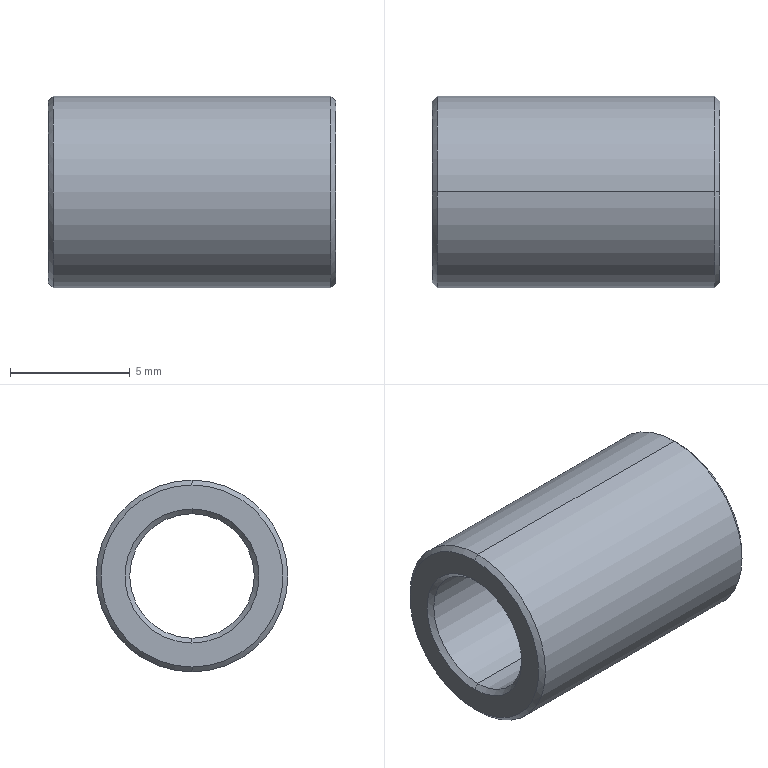Part | NX | features BREP 1 | 1 solid | 14 faces | box 12 x 8 x 8 mm | volume 346.681 mm3 | cone 8 | cylinder 4 | plane 2 | commonest cylinder face diameters 5.2 x2 8 x2
STEP:
#1=CARTESIAN_POINT('',(11.8,0.,-4.));
#2=VERTEX_POINT('',#1);
#3=CARTESIAN_POINT('',(12.,0.,-3.8));
#4=VERTEX_POINT('',#3);
#5=CARTESIAN_POINT('',(12.,0.,-3.8));
#6=DIRECTION('',(-0.7071,0.,-0.7071));
#7=VECTOR('',#6,1000.);
#8=LINE('',#5,#7);
#9=EDGE_CURVE('',#2,#4,#8,.F.);
#10=ORIENTED_EDGE('',*,*,#9,.T.);
#11=CARTESIAN_POINT('',(12.,0.,3.8));
#12=VERTEX_POINT('',#11);
#13=CARTESIAN_POINT('',(12.,0.,0.));
#14=DIRECTION('',(1.,0.,0.));
#15=DIRECTION('',(0.,0.,-1.));
#16=AXIS2_PLACEMENT_3D('',#13,#14,#15);
#17=CIRCLE('',#16,3.8);
#18=EDGE_CURVE('',#12,#4,#17,.T.);
#19=ORIENTED_EDGE('',*,*,#18,.F.);
#20=CARTESIAN_POINT('',(11.8,0.,4.));
#21=VERTEX_POINT('',#20);
#22=CARTESIAN_POINT('',(12.,0.,3.8));
#23=DIRECTION('',(-0.7071,0.,0.7071));
#24=VECTOR('',#23,1000.);
#25=LINE('',#22,#24);
#26=EDGE_CURVE('',#21,#12,#25,.F.);
#27=ORIENTED_EDGE('',*,*,#26,.F.);
#28=CARTESIAN_POINT('',(11.8,0.,0.));
#29=DIRECTION('',(-1.,0.,0.));
#30=DIRECTION('',(0.,0.,-1.));
#31=AXIS2_PLACEMENT_3D('',#28,#29,#30);
#32=CIRCLE('',#31,4.);
#33=EDGE_CURVE('',#2,#21,#32,.T.);
#34=ORIENTED_EDGE('',*,*,#33,.F.);
#35=EDGE_LOOP('',(#10,#19,#27,#34));
#36=FACE_BOUND('',#35,.T.);
#37=CARTESIAN_POINT('',(12.,0.,0.));
#38=DIRECTION('',(-1.,0.,0.));
#39=DIRECTION('',(0.,0.,1.));
#40=AXIS2_PLACEMENT_3D('',#37,#38,#39);
#41=CONICAL_SURFACE('',#40,3.8,0.7854);
#42=ADVANCED_FACE('',(#36),#41,.T.);
#43=CARTESIAN_POINT('',(11.8,0.,2.6));
#44=VERTEX_POINT('',#43);
#45=CARTESIAN_POINT('',(12.,0.,2.8));
#46=VERTEX_POINT('',#45);
#47=CARTESIAN_POINT('',(11.8,0.,2.6));
#48=DIRECTION('',(0.7071,0.,0.7071));
#49=VECTOR('',#48,1000.);
#50=LINE('',#47,#49);
#51=EDGE_CURVE('',#44,#46,#50,.T.);
#52=ORIENTED_EDGE('',*,*,#51,.F.);
#53=CARTESIAN_POINT('',(11.8,0.,-2.6));
#54=VERTEX_POINT('',#53);
#55=CARTESIAN_POINT('',(11.8,0.,0.));
#56=DIRECTION('',(1.,0.,0.));
#57=DIRECTION('',(0.,0.,-1.));
#58=AXIS2_PLACEMENT_3D('',#55,#56,#57);
#59=CIRCLE('',#58,2.6);
#60=EDGE_CURVE('',#54,#44,#59,.T.);
#61=ORIENTED_EDGE('',*,*,#60,.F.);
#62=CARTESIAN_POINT('',(12.,0.,-2.8));
#63=VERTEX_POINT('',#62);
#64=CARTESIAN_POINT('',(11.8,0.,-2.6));
#65=DIRECTION('',(0.7071,0.,-0.7071));
#66=VECTOR('',#65,1000.);
#67=LINE('',#64,#66);
#68=EDGE_CURVE('',#54,#63,#67,.T.);
#69=ORIENTED_EDGE('',*,*,#68,.T.);
#70=CARTESIAN_POINT('',(12.,0.,0.));
#71=DIRECTION('',(-1.,0.,0.));
#72=DIRECTION('',(0.,0.,-1.));
#73=AXIS2_PLACEMENT_3D('',#70,#71,#72);
#74=CIRCLE('',#73,2.8);
#75=EDGE_CURVE('',#46,#63,#74,.T.);
#76=ORIENTED_EDGE('',*,*,#75,.F.);
#77=EDGE_LOOP('',(#52,#61,#69,#76));
#78=FACE_BOUND('',#77,.T.);
#79=CARTESIAN_POINT('',(11.8,0.,0.));
#80=DIRECTION('',(1.,0.,0.));
#81=DIRECTION('',(0.,0.,-1.));
#82=AXIS2_PLACEMENT_3D('',#79,#80,#81);
#83=CONICAL_SURFACE('',#82,2.6,0.7854);
#84=ADVANCED_FACE('',(#78),#83,.F.);
#85=CARTESIAN_POINT('',(0.,0.,3.8));
#86=VERTEX_POINT('',#85);
#87=CARTESIAN_POINT('',(0.2,0.,4.));
#88=VERTEX_POINT('',#87);
#89=CARTESIAN_POINT('',(0.2,0.,4.));
#90=DIRECTION('',(0.7071,0.,0.7071));
#91=VECTOR('',#90,1000.);
#92=LINE('',#89,#91);
#93=EDGE_CURVE('',#86,#88,#92,.T.);
#94=ORIENTED_EDGE('',*,*,#93,.F.);
#95=CARTESIAN_POINT('',(0.,0.,-3.8));
#96=VERTEX_POINT('',#95);
#97=CARTESIAN_POINT('',(0.,0.,0.));
#98=DIRECTION('',(-1.,0.,0.));
#99=DIRECTION('',(0.,0.,-1.));
#100=AXIS2_PLACEMENT_3D('',#97,#98,#99);
#101=CIRCLE('',#100,3.8);
#102=EDGE_CURVE('',#96,#86,#101,.T.);
#103=ORIENTED_EDGE('',*,*,#102,.F.);
#104=CARTESIAN_POINT('',(0.2,0.,-4.));
#105=VERTEX_POINT('',#104);
#106=CARTESIAN_POINT('',(0.2,0.,-4.));
#107=DIRECTION('',(0.7071,0.,-0.7071));
#108=VECTOR('',#107,1000.);
#109=LINE('',#106,#108);
#110=EDGE_CURVE('',#96,#105,#109,.T.);
#111=ORIENTED_EDGE('',*,*,#110,.T.);
#112=CARTESIAN_POINT('',(0.2,0.,0.));
#113=DIRECTION('',(1.,0.,0.));
#114=DIRECTION('',(0.,0.,-1.));
#115=AXIS2_PLACEMENT_3D('',#112,#113,#114);
#116=CIRCLE('',#115,4.);
#117=EDGE_CURVE('',#88,#105,#116,.T.);
#118=ORIENTED_EDGE('',*,*,#117,.F.);
#119=EDGE_LOOP('',(#94,#103,#111,#118));
#120=FACE_BOUND('',#119,.T.);
#121=CARTESIAN_POINT('',(0.2,0.,0.));
#122=DIRECTION('',(1.,0.,0.));
#123=DIRECTION('',(0.,0.,-1.));
#124=AXIS2_PLACEMENT_3D('',#121,#122,#123);
#125=CONICAL_SURFACE('',#124,4.,0.7854);
#126=ADVANCED_FACE('',(#120),#125,.T.);
#127=CARTESIAN_POINT('',(0.,0.,-2.8));
#128=VERTEX_POINT('',#127);
#129=CARTESIAN_POINT('',(0.2,0.,-2.6));
#130=VERTEX_POINT('',#129);
#131=CARTESIAN_POINT('',(0.,0.,-2.8));
#132=DIRECTION('',(-0.7071,0.,-0.7071));
#133=VECTOR('',#132,1000.);
#134=LINE('',#131,#133);
#135=EDGE_CURVE('',#128,#130,#134,.F.);
#136=ORIENTED_EDGE('',*,*,#135,.T.);
#137=CARTESIAN_POINT('',(0.2,0.,2.6));
#138=VERTEX_POINT('',#137);
#139=CARTESIAN_POINT('',(0.2,0.,0.));
#140=DIRECTION('',(-1.,0.,0.));
#141=DIRECTION('',(0.,0.,-1.));
#142=AXIS2_PLACEMENT_3D('',#139,#140,#141);
#143=CIRCLE('',#142,2.6);
#144=EDGE_CURVE('',#138,#130,#143,.T.);
#145=ORIENTED_EDGE('',*,*,#144,.F.);
#146=CARTESIAN_POINT('',(0.,0.,2.8));
#147=VERTEX_POINT('',#146);
#148=CARTESIAN_POINT('',(0.,0.,2.8));
#149=DIRECTION('',(-0.7071,0.,0.7071));
#150=VECTOR('',#149,1000.);
#151=LINE('',#148,#150);
#152=EDGE_CURVE('',#147,#138,#151,.F.);
#153=ORIENTED_EDGE('',*,*,#152,.F.);
#154=CARTESIAN_POINT('',(0.,0.,0.));
#155=DIRECTION('',(1.,0.,0.));
#156=DIRECTION('',(0.,0.,-1.));
#157=AXIS2_PLACEMENT_3D('',#154,#155,#156);
#158=CIRCLE('',#157,2.8);
#159=EDGE_CURVE('',#128,#147,#158,.T.);
#160=ORIENTED_EDGE('',*,*,#159,.F.);
#161=EDGE_LOOP('',(#136,#145,#153,#160));
#162=FACE_BOUND('',#161,.T.);
#163=CARTESIAN_POINT('',(0.,0.,0.));
#164=DIRECTION('',(-1.,0.,0.));
#165=DIRECTION('',(0.,0.,1.));
#166=AXIS2_PLACEMENT_3D('',#163,#164,#165);
#167=CONICAL_SURFACE('',#166,2.8,0.7854);
#168=ADVANCED_FACE('',(#162),#167,.F.);
#169=CARTESIAN_POINT('',(12.,0.,-2.6));
#170=DIRECTION('',(-1.,0.,0.));
#171=VECTOR('',#170,1000.);
#172=LINE('',#169,#171);
#173=EDGE_CURVE('',#130,#54,#172,.F.);
#174=ORIENTED_EDGE('',*,*,#173,.T.);
#175=ORIENTED_EDGE('',*,*,#60,.T.);
#176=CARTESIAN_POINT('',(12.,0.,2.6));
#177=DIRECTION('',(-1.,0.,0.));
#178=VECTOR('',#177,1000.);
#179=LINE('',#176,#178);
#180=EDGE_CURVE('',#138,#44,#179,.F.);
#181=ORIENTED_EDGE('',*,*,#180,.F.);
#182=ORIENTED_EDGE('',*,*,#144,.T.);
#183=EDGE_LOOP('',(#174,#175,#181,#182));
#184=FACE_BOUND('',#183,.T.);
#185=CARTESIAN_POINT('',(12.,0.,0.));
#186=DIRECTION('',(-1.,0.,0.));
#187=DIRECTION('',(0.,0.,1.));
#188=AXIS2_PLACEMENT_3D('',#185,#186,#187);
#189=CYLINDRICAL_SURFACE('',#188,2.6);
#190=ADVANCED_FACE('',(#184),#189,.F.);
#191=CARTESIAN_POINT('',(12.,0.,-4.));
#192=DIRECTION('',(-1.,0.,0.));
#193=VECTOR('',#192,1000.);
#194=LINE('',#191,#193);
#195=EDGE_CURVE('',#105,#2,#194,.F.);
#196=ORIENTED_EDGE('',*,*,#195,.T.);
#197=ORIENTED_EDGE('',*,*,#33,.T.);
#198=CARTESIAN_POINT('',(12.,0.,4.));
#199=DIRECTION('',(-1.,0.,0.));
#200=VECTOR('',#199,1000.);
#201=LINE('',#198,#200);
#202=EDGE_CURVE('',#88,#21,#201,.F.);
#203=ORIENTED_EDGE('',*,*,#202,.F.);
#204=ORIENTED_EDGE('',*,*,#117,.T.);
#205=EDGE_LOOP('',(#196,#197,#203,#204));
#206=FACE_BOUND('',#205,.T.);
#207=CARTESIAN_POINT('',(12.,0.,0.));
#208=DIRECTION('',(-1.,0.,0.));
#209=DIRECTION('',(0.,0.,1.));
#210=AXIS2_PLACEMENT_3D('',#207,#208,#209);
#211=CYLINDRICAL_SURFACE('',#210,4.);
#212=ADVANCED_FACE('',(#206),#211,.T.);
#213=ORIENTED_EDGE('',*,*,#102,.T.);
#214=CARTESIAN_POINT('',(0.,0.,0.));
#215=DIRECTION('',(-1.,0.,0.));
#216=DIRECTION('',(0.,0.,-1.));
#217=AXIS2_PLACEMENT_3D('',#214,#215,#216);
#218=CIRCLE('',#217,3.8);
#219=EDGE_CURVE('',#86,#96,#218,.T.);
#220=ORIENTED_EDGE('',*,*,#219,.T.);
#221=EDGE_LOOP('',(#213,#220));
#222=FACE_BOUND('',#221,.T.);
#223=CARTESIAN_POINT('',(0.,0.,0.));
#224=DIRECTION('',(1.,0.,0.));
#225=DIRECTION('',(0.,0.,-1.));
#226=AXIS2_PLACEMENT_3D('',#223,#224,#225);
#227=CIRCLE('',#226,2.8);
#228=EDGE_CURVE('',#147,#128,#227,.T.);
#229=ORIENTED_EDGE('',*,*,#228,.T.);
#230=ORIENTED_EDGE('',*,*,#159,.T.);
#231=EDGE_LOOP('',(#229,#230));
#232=FACE_BOUND('',#231,.T.);
#233=CARTESIAN_POINT('',(0.,0.,0.));
#234=DIRECTION('',(1.,0.,0.));
#235=DIRECTION('',(0.,0.,-1.));
#236=AXIS2_PLACEMENT_3D('',#233,#234,#235);
#237=PLANE('',#236);
#238=ADVANCED_FACE('',(#222,#232),#237,.F.);
#239=ORIENTED_EDGE('',*,*,#18,.T.);
#240=CARTESIAN_POINT('',(12.,0.,0.));
#241=DIRECTION('',(1.,0.,0.));
#242=DIRECTION('',(0.,0.,-1.));
#243=AXIS2_PLACEMENT_3D('',#240,#241,#242);
#244=CIRCLE('',#243,3.8);
#245=EDGE_CURVE('',#4,#12,#244,.T.);
#246=ORIENTED_EDGE('',*,*,#245,.T.);
#247=EDGE_LOOP('',(#239,#246));
#248=FACE_BOUND('',#247,.T.);
#249=CARTESIAN_POINT('',(12.,0.,0.));
#250=DIRECTION('',(-1.,0.,0.));
#251=DIRECTION('',(0.,0.,-1.));
#252=AXIS2_PLACEMENT_3D('',#249,#250,#251);
#253=CIRCLE('',#252,2.8);
#254=EDGE_CURVE('',#63,#46,#253,.T.);
#255=ORIENTED_EDGE('',*,*,#254,.T.);
#256=ORIENTED_EDGE('',*,*,#75,.T.);
#257=EDGE_LOOP('',(#255,#256));
#258=FACE_BOUND('',#257,.T.);
#259=CARTESIAN_POINT('',(12.,0.,0.));
#260=DIRECTION('',(1.,0.,0.));
#261=DIRECTION('',(0.,0.,-1.));
#262=AXIS2_PLACEMENT_3D('',#259,#260,#261);
#263=PLANE('',#262);
#264=ADVANCED_FACE('',(#248,#258),#263,.T.);
#265=CARTESIAN_POINT('',(11.8,0.,0.));
#266=DIRECTION('',(-1.,0.,0.));
#267=DIRECTION('',(0.,0.,-1.));
#268=AXIS2_PLACEMENT_3D('',#265,#266,#267);
#269=CIRCLE('',#268,4.);
#270=EDGE_CURVE('',#21,#2,#269,.T.);
#271=ORIENTED_EDGE('',*,*,#270,.T.);
#272=ORIENTED_EDGE('',*,*,#195,.F.);
#273=CARTESIAN_POINT('',(0.2,0.,0.));
#274=DIRECTION('',(1.,0.,0.));
#275=DIRECTION('',(0.,0.,-1.));
#276=AXIS2_PLACEMENT_3D('',#273,#274,#275);
#277=CIRCLE('',#276,4.);
#278=EDGE_CURVE('',#105,#88,#277,.T.);
#279=ORIENTED_EDGE('',*,*,#278,.T.);
#280=ORIENTED_EDGE('',*,*,#202,.T.);
#281=EDGE_LOOP('',(#271,#272,#279,#280));
#282=FACE_BOUND('',#281,.T.);
#283=CARTESIAN_POINT('',(12.,0.,0.));
#284=DIRECTION('',(-1.,0.,0.));
#285=DIRECTION('',(0.,0.,1.));
#286=AXIS2_PLACEMENT_3D('',#283,#284,#285);
#287=CYLINDRICAL_SURFACE('',#286,4.);
#288=ADVANCED_FACE('',(#282),#287,.T.);
#289=CARTESIAN_POINT('',(11.8,0.,0.));
#290=DIRECTION('',(1.,0.,0.));
#291=DIRECTION('',(0.,0.,-1.));
#292=AXIS2_PLACEMENT_3D('',#289,#290,#291);
#293=CIRCLE('',#292,2.6);
#294=EDGE_CURVE('',#44,#54,#293,.T.);
#295=ORIENTED_EDGE('',*,*,#294,.T.);
#296=ORIENTED_EDGE('',*,*,#173,.F.);
#297=CARTESIAN_POINT('',(0.2,0.,0.));
#298=DIRECTION('',(-1.,0.,0.));
#299=DIRECTION('',(0.,0.,-1.));
#300=AXIS2_PLACEMENT_3D('',#297,#298,#299);
#301=CIRCLE('',#300,2.6);
#302=EDGE_CURVE('',#130,#138,#301,.T.);
#303=ORIENTED_EDGE('',*,*,#302,.T.);
#304=ORIENTED_EDGE('',*,*,#180,.T.);
#305=EDGE_LOOP('',(#295,#296,#303,#304));
#306=FACE_BOUND('',#305,.T.);
#307=CARTESIAN_POINT('',(12.,0.,0.));
#308=DIRECTION('',(-1.,0.,0.));
#309=DIRECTION('',(0.,0.,1.));
#310=AXIS2_PLACEMENT_3D('',#307,#308,#309);
#311=CYLINDRICAL_SURFACE('',#310,2.6);
#312=ADVANCED_FACE('',(#306),#311,.F.);
#313=ORIENTED_EDGE('',*,*,#302,.F.);
#314=ORIENTED_EDGE('',*,*,#135,.F.);
#315=ORIENTED_EDGE('',*,*,#228,.F.);
#316=ORIENTED_EDGE('',*,*,#152,.T.);
#317=EDGE_LOOP('',(#313,#314,#315,#316));
#318=FACE_BOUND('',#317,.T.);
#319=CARTESIAN_POINT('',(0.,0.,0.));
#320=DIRECTION('',(-1.,0.,0.));
#321=DIRECTION('',(0.,0.,1.));
#322=AXIS2_PLACEMENT_3D('',#319,#320,#321);
#323=CONICAL_SURFACE('',#322,2.8,0.7854);
#324=ADVANCED_FACE('',(#318),#323,.F.);
#325=ORIENTED_EDGE('',*,*,#219,.F.);
#326=ORIENTED_EDGE('',*,*,#93,.T.);
#327=ORIENTED_EDGE('',*,*,#278,.F.);
#328=ORIENTED_EDGE('',*,*,#110,.F.);
#329=EDGE_LOOP('',(#325,#326,#327,#328));
#330=FACE_BOUND('',#329,.T.);
#331=CARTESIAN_POINT('',(0.2,0.,0.));
#332=DIRECTION('',(1.,0.,0.));
#333=DIRECTION('',(0.,0.,-1.));
#334=AXIS2_PLACEMENT_3D('',#331,#332,#333);
#335=CONICAL_SURFACE('',#334,4.,0.7854);
#336=ADVANCED_FACE('',(#330),#335,.T.);
#337=ORIENTED_EDGE('',*,*,#294,.F.);
#338=ORIENTED_EDGE('',*,*,#51,.T.);
#339=ORIENTED_EDGE('',*,*,#254,.F.);
#340=ORIENTED_EDGE('',*,*,#68,.F.);
#341=EDGE_LOOP('',(#337,#338,#339,#340));
#342=FACE_BOUND('',#341,.T.);
#343=CARTESIAN_POINT('',(11.8,0.,0.));
#344=DIRECTION('',(1.,0.,0.));
#345=DIRECTION('',(0.,0.,-1.));
#346=AXIS2_PLACEMENT_3D('',#343,#344,#345);
#347=CONICAL_SURFACE('',#346,2.6,0.7854);
#348=ADVANCED_FACE('',(#342),#347,.F.);
#349=ORIENTED_EDGE('',*,*,#245,.F.);
#350=ORIENTED_EDGE('',*,*,#9,.F.);
#351=ORIENTED_EDGE('',*,*,#270,.F.);
#352=ORIENTED_EDGE('',*,*,#26,.T.);
#353=EDGE_LOOP('',(#349,#350,#351,#352));
#354=FACE_BOUND('',#353,.T.);
#355=CARTESIAN_POINT('',(12.,0.,0.));
#356=DIRECTION('',(-1.,0.,0.));
#357=DIRECTION('',(0.,0.,1.));
#358=AXIS2_PLACEMENT_3D('',#355,#356,#357);
#359=CONICAL_SURFACE('',#358,3.8,0.7854);
#360=ADVANCED_FACE('',(#354),#359,.T.);
#361=CLOSED_SHELL('',(#42,#84,#126,#168,#190,#212,#238,#264,#288,#312,#324,#336,#348,#360));
#362=MANIFOLD_SOLID_BREP('',#361);
#363=(LENGTH_UNIT()NAMED_UNIT(*)SI_UNIT(.MILLI.,.METRE.));
#364=UNCERTAINTY_MEASURE_WITH_UNIT(LENGTH_MEASURE(0.00001),#363,'','');
#365=(NAMED_UNIT(*)PLANE_ANGLE_UNIT()SI_UNIT($,.RADIAN.));
#366=(NAMED_UNIT(*)SI_UNIT($,.STERADIAN.)SOLID_ANGLE_UNIT());
#367=(GEOMETRIC_REPRESENTATION_CONTEXT(3)GLOBAL_UNCERTAINTY_ASSIGNED_CONTEXT((#364))GLOBAL_UNIT_ASSIGNED_CONTEXT((#363,#365,#366))REPRESENTATION_CONTEXT('',''));
#368=ADVANCED_BREP_SHAPE_REPRESENTATION('',(#362),#367);